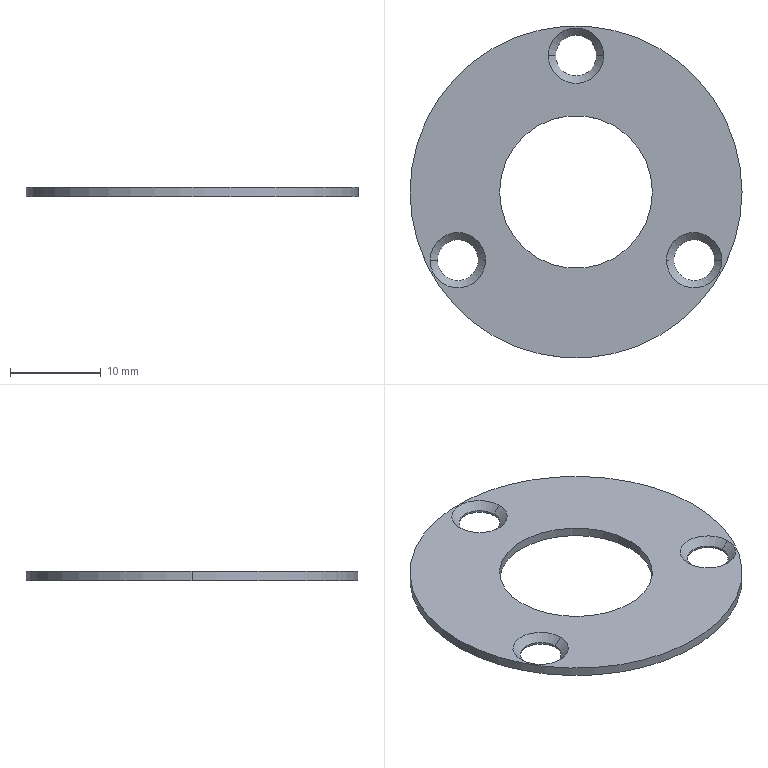Part | SolidWorks | features Chamfer 1, Extrusion 1 | 1 solid | 18 faces | box 36.5 x 36.5 x 1 mm | volume 761.783 mm3 | cylinder 10 | cone 6 | plane 2 | commonest cylinder face diameters 4.5 x6 16.8 x2 36.5 x2
STEP:
#1=CARTESIAN_POINT('',(-2.25,15.,0.2));
#2=VERTEX_POINT('',#1);
#3=CARTESIAN_POINT('',(2.25,15.,0.2));
#4=VERTEX_POINT('',#3);
#5=CARTESIAN_POINT('',(0.,15.,0.2));
#6=DIRECTION('',(0.,0.,1.));
#7=DIRECTION('',(1.,0.,0.));
#8=AXIS2_PLACEMENT_3D('',#5,#6,#7);
#9=CIRCLE('',#8,2.25);
#10=EDGE_CURVE('',#2,#4,#9,.T.);
#11=ORIENTED_EDGE('',*,*,#10,.F.);
#12=CARTESIAN_POINT('',(-3.05,15.,1.));
#13=VERTEX_POINT('',#12);
#14=CARTESIAN_POINT('',(-2.25,15.,0.2));
#15=DIRECTION('',(-0.7071,0.,0.7071));
#16=VECTOR('',#15,1000.);
#17=LINE('',#14,#16);
#18=EDGE_CURVE('',#2,#13,#17,.T.);
#19=ORIENTED_EDGE('',*,*,#18,.T.);
#20=CARTESIAN_POINT('',(3.05,15.,1.));
#21=VERTEX_POINT('',#20);
#22=CARTESIAN_POINT('',(0.,15.,1.));
#23=DIRECTION('',(0.,0.,-1.));
#24=DIRECTION('',(1.,0.,0.));
#25=AXIS2_PLACEMENT_3D('',#22,#23,#24);
#26=CIRCLE('',#25,3.05);
#27=EDGE_CURVE('',#21,#13,#26,.T.);
#28=ORIENTED_EDGE('',*,*,#27,.F.);
#29=CARTESIAN_POINT('',(2.25,15.,0.2));
#30=DIRECTION('',(0.7071,0.,0.7071));
#31=VECTOR('',#30,1000.);
#32=LINE('',#29,#31);
#33=EDGE_CURVE('',#4,#21,#32,.T.);
#34=ORIENTED_EDGE('',*,*,#33,.F.);
#35=EDGE_LOOP('',(#11,#19,#28,#34));
#36=FACE_OUTER_BOUND('',#35,.T.);
#37=CARTESIAN_POINT('',(0.,15.,0.2));
#38=DIRECTION('',(0.,0.,1.));
#39=DIRECTION('',(1.,0.,0.));
#40=AXIS2_PLACEMENT_3D('',#37,#38,#39);
#41=CONICAL_SURFACE('',#40,2.25,0.7854);
#42=ADVANCED_FACE('',(#36),#41,.F.);
#43=CARTESIAN_POINT('',(-15.24,-7.5,0.2));
#44=VERTEX_POINT('',#43);
#45=CARTESIAN_POINT('',(-10.74,-7.5,0.2));
#46=VERTEX_POINT('',#45);
#47=CARTESIAN_POINT('',(-12.99,-7.5,0.2));
#48=DIRECTION('',(0.,0.,1.));
#49=DIRECTION('',(1.,0.,0.));
#50=AXIS2_PLACEMENT_3D('',#47,#48,#49);
#51=CIRCLE('',#50,2.25);
#52=EDGE_CURVE('',#44,#46,#51,.T.);
#53=ORIENTED_EDGE('',*,*,#52,.F.);
#54=CARTESIAN_POINT('',(-16.04,-7.5,1.));
#55=VERTEX_POINT('',#54);
#56=CARTESIAN_POINT('',(-15.24,-7.5,0.2));
#57=DIRECTION('',(-0.7071,0.,0.7071));
#58=VECTOR('',#57,1000.);
#59=LINE('',#56,#58);
#60=EDGE_CURVE('',#44,#55,#59,.T.);
#61=ORIENTED_EDGE('',*,*,#60,.T.);
#62=CARTESIAN_POINT('',(-9.94,-7.5,1.));
#63=VERTEX_POINT('',#62);
#64=CARTESIAN_POINT('',(-12.99,-7.5,1.));
#65=DIRECTION('',(0.,0.,-1.));
#66=DIRECTION('',(1.,0.,0.));
#67=AXIS2_PLACEMENT_3D('',#64,#65,#66);
#68=CIRCLE('',#67,3.05);
#69=EDGE_CURVE('',#63,#55,#68,.T.);
#70=ORIENTED_EDGE('',*,*,#69,.F.);
#71=CARTESIAN_POINT('',(-10.74,-7.5,0.2));
#72=DIRECTION('',(0.7071,0.,0.7071));
#73=VECTOR('',#72,1000.);
#74=LINE('',#71,#73);
#75=EDGE_CURVE('',#46,#63,#74,.T.);
#76=ORIENTED_EDGE('',*,*,#75,.F.);
#77=EDGE_LOOP('',(#53,#61,#70,#76));
#78=FACE_OUTER_BOUND('',#77,.T.);
#79=CARTESIAN_POINT('',(-12.99,-7.5,0.2));
#80=DIRECTION('',(0.,0.,1.));
#81=DIRECTION('',(1.,0.,0.));
#82=AXIS2_PLACEMENT_3D('',#79,#80,#81);
#83=CONICAL_SURFACE('',#82,2.25,0.7854);
#84=ADVANCED_FACE('',(#78),#83,.F.);
#85=CARTESIAN_POINT('',(10.74,-7.5,0.2));
#86=VERTEX_POINT('',#85);
#87=CARTESIAN_POINT('',(15.24,-7.5,0.2));
#88=VERTEX_POINT('',#87);
#89=CARTESIAN_POINT('',(12.99,-7.5,0.2));
#90=DIRECTION('',(0.,0.,1.));
#91=DIRECTION('',(1.,0.,0.));
#92=AXIS2_PLACEMENT_3D('',#89,#90,#91);
#93=CIRCLE('',#92,2.25);
#94=EDGE_CURVE('',#86,#88,#93,.T.);
#95=ORIENTED_EDGE('',*,*,#94,.F.);
#96=CARTESIAN_POINT('',(9.94,-7.5,1.));
#97=VERTEX_POINT('',#96);
#98=CARTESIAN_POINT('',(10.74,-7.5,0.2));
#99=DIRECTION('',(-0.7071,0.,0.7071));
#100=VECTOR('',#99,1000.);
#101=LINE('',#98,#100);
#102=EDGE_CURVE('',#86,#97,#101,.T.);
#103=ORIENTED_EDGE('',*,*,#102,.T.);
#104=CARTESIAN_POINT('',(16.04,-7.5,1.));
#105=VERTEX_POINT('',#104);
#106=CARTESIAN_POINT('',(12.99,-7.5,1.));
#107=DIRECTION('',(0.,0.,-1.));
#108=DIRECTION('',(1.,0.,0.));
#109=AXIS2_PLACEMENT_3D('',#106,#107,#108);
#110=CIRCLE('',#109,3.05);
#111=EDGE_CURVE('',#105,#97,#110,.T.);
#112=ORIENTED_EDGE('',*,*,#111,.F.);
#113=CARTESIAN_POINT('',(15.24,-7.5,0.2));
#114=DIRECTION('',(0.7071,0.,0.7071));
#115=VECTOR('',#114,1000.);
#116=LINE('',#113,#115);
#117=EDGE_CURVE('',#88,#105,#116,.T.);
#118=ORIENTED_EDGE('',*,*,#117,.F.);
#119=EDGE_LOOP('',(#95,#103,#112,#118));
#120=FACE_OUTER_BOUND('',#119,.T.);
#121=CARTESIAN_POINT('',(12.99,-7.5,0.2));
#122=DIRECTION('',(0.,0.,1.));
#123=DIRECTION('',(1.,0.,0.));
#124=AXIS2_PLACEMENT_3D('',#121,#122,#123);
#125=CONICAL_SURFACE('',#124,2.25,0.7854);
#126=ADVANCED_FACE('',(#120),#125,.F.);
#127=ORIENTED_EDGE('',*,*,#52,.T.);
#128=CARTESIAN_POINT('',(-10.74,-7.5,0.));
#129=VERTEX_POINT('',#128);
#130=CARTESIAN_POINT('',(-10.74,-7.5,1.));
#131=DIRECTION('',(0.,0.,-1.));
#132=VECTOR('',#131,1000.);
#133=LINE('',#130,#132);
#134=EDGE_CURVE('',#46,#129,#133,.T.);
#135=ORIENTED_EDGE('',*,*,#134,.T.);
#136=CARTESIAN_POINT('',(-15.24,-7.5,0.));
#137=VERTEX_POINT('',#136);
#138=CARTESIAN_POINT('',(-12.99,-7.5,0.));
#139=DIRECTION('',(0.,0.,1.));
#140=DIRECTION('',(1.,0.,0.));
#141=AXIS2_PLACEMENT_3D('',#138,#139,#140);
#142=CIRCLE('',#141,2.25);
#143=EDGE_CURVE('',#137,#129,#142,.T.);
#144=ORIENTED_EDGE('',*,*,#143,.F.);
#145=CARTESIAN_POINT('',(-15.24,-7.5,1.));
#146=DIRECTION('',(0.,0.,-1.));
#147=VECTOR('',#146,1000.);
#148=LINE('',#145,#147);
#149=EDGE_CURVE('',#44,#137,#148,.T.);
#150=ORIENTED_EDGE('',*,*,#149,.F.);
#151=EDGE_LOOP('',(#127,#135,#144,#150));
#152=FACE_OUTER_BOUND('',#151,.T.);
#153=CARTESIAN_POINT('',(-12.99,-7.5,1.));
#154=DIRECTION('',(0.,0.,-1.));
#155=DIRECTION('',(-1.,0.,0.));
#156=AXIS2_PLACEMENT_3D('',#153,#154,#155);
#157=CYLINDRICAL_SURFACE('',#156,2.25);
#158=ADVANCED_FACE('',(#152),#157,.F.);
#159=ORIENTED_EDGE('',*,*,#94,.T.);
#160=CARTESIAN_POINT('',(15.24,-7.5,0.));
#161=VERTEX_POINT('',#160);
#162=CARTESIAN_POINT('',(15.24,-7.5,1.));
#163=DIRECTION('',(0.,0.,-1.));
#164=VECTOR('',#163,1000.);
#165=LINE('',#162,#164);
#166=EDGE_CURVE('',#88,#161,#165,.T.);
#167=ORIENTED_EDGE('',*,*,#166,.T.);
#168=CARTESIAN_POINT('',(10.74,-7.5,0.));
#169=VERTEX_POINT('',#168);
#170=CARTESIAN_POINT('',(12.99,-7.5,0.));
#171=DIRECTION('',(0.,0.,1.));
#172=DIRECTION('',(1.,0.,0.));
#173=AXIS2_PLACEMENT_3D('',#170,#171,#172);
#174=CIRCLE('',#173,2.25);
#175=EDGE_CURVE('',#169,#161,#174,.T.);
#176=ORIENTED_EDGE('',*,*,#175,.F.);
#177=CARTESIAN_POINT('',(10.74,-7.5,1.));
#178=DIRECTION('',(0.,0.,-1.));
#179=VECTOR('',#178,1000.);
#180=LINE('',#177,#179);
#181=EDGE_CURVE('',#86,#169,#180,.T.);
#182=ORIENTED_EDGE('',*,*,#181,.F.);
#183=EDGE_LOOP('',(#159,#167,#176,#182));
#184=FACE_OUTER_BOUND('',#183,.T.);
#185=CARTESIAN_POINT('',(12.99,-7.5,1.));
#186=DIRECTION('',(0.,0.,-1.));
#187=DIRECTION('',(-1.,0.,0.));
#188=AXIS2_PLACEMENT_3D('',#185,#186,#187);
#189=CYLINDRICAL_SURFACE('',#188,2.25);
#190=ADVANCED_FACE('',(#184),#189,.F.);
#191=ORIENTED_EDGE('',*,*,#10,.T.);
#192=CARTESIAN_POINT('',(2.25,15.,0.));
#193=VERTEX_POINT('',#192);
#194=CARTESIAN_POINT('',(2.25,15.,1.));
#195=DIRECTION('',(0.,0.,-1.));
#196=VECTOR('',#195,1000.);
#197=LINE('',#194,#196);
#198=EDGE_CURVE('',#4,#193,#197,.T.);
#199=ORIENTED_EDGE('',*,*,#198,.T.);
#200=CARTESIAN_POINT('',(-2.25,15.,0.));
#201=VERTEX_POINT('',#200);
#202=CARTESIAN_POINT('',(0.,15.,0.));
#203=DIRECTION('',(0.,0.,1.));
#204=DIRECTION('',(1.,0.,0.));
#205=AXIS2_PLACEMENT_3D('',#202,#203,#204);
#206=CIRCLE('',#205,2.25);
#207=EDGE_CURVE('',#201,#193,#206,.T.);
#208=ORIENTED_EDGE('',*,*,#207,.F.);
#209=CARTESIAN_POINT('',(-2.25,15.,1.));
#210=DIRECTION('',(0.,0.,-1.));
#211=VECTOR('',#210,1000.);
#212=LINE('',#209,#211);
#213=EDGE_CURVE('',#2,#201,#212,.T.);
#214=ORIENTED_EDGE('',*,*,#213,.F.);
#215=EDGE_LOOP('',(#191,#199,#208,#214));
#216=FACE_OUTER_BOUND('',#215,.T.);
#217=CARTESIAN_POINT('',(0.,15.,1.));
#218=DIRECTION('',(0.,0.,-1.));
#219=DIRECTION('',(-1.,0.,0.));
#220=AXIS2_PLACEMENT_3D('',#217,#218,#219);
#221=CYLINDRICAL_SURFACE('',#220,2.25);
#222=ADVANCED_FACE('',(#216),#221,.F.);
#223=CARTESIAN_POINT('',(-8.4,0.,1.));
#224=VERTEX_POINT('',#223);
#225=CARTESIAN_POINT('',(8.4,0.,1.));
#226=VERTEX_POINT('',#225);
#227=CARTESIAN_POINT('',(0.,0.,1.));
#228=DIRECTION('',(0.,0.,1.));
#229=DIRECTION('',(1.,0.,0.));
#230=AXIS2_PLACEMENT_3D('',#227,#228,#229);
#231=CIRCLE('',#230,8.4);
#232=EDGE_CURVE('',#224,#226,#231,.T.);
#233=ORIENTED_EDGE('',*,*,#232,.T.);
#234=CARTESIAN_POINT('',(8.4,0.,0.));
#235=VERTEX_POINT('',#234);
#236=CARTESIAN_POINT('',(8.4,0.,1.));
#237=DIRECTION('',(0.,0.,-1.));
#238=VECTOR('',#237,1000.);
#239=LINE('',#236,#238);
#240=EDGE_CURVE('',#226,#235,#239,.T.);
#241=ORIENTED_EDGE('',*,*,#240,.T.);
#242=CARTESIAN_POINT('',(-8.4,0.,0.));
#243=VERTEX_POINT('',#242);
#244=CARTESIAN_POINT('',(0.,0.,0.));
#245=DIRECTION('',(0.,0.,1.));
#246=DIRECTION('',(1.,0.,0.));
#247=AXIS2_PLACEMENT_3D('',#244,#245,#246);
#248=CIRCLE('',#247,8.4);
#249=EDGE_CURVE('',#243,#235,#248,.T.);
#250=ORIENTED_EDGE('',*,*,#249,.F.);
#251=CARTESIAN_POINT('',(-8.4,0.,1.));
#252=DIRECTION('',(0.,0.,-1.));
#253=VECTOR('',#252,1000.);
#254=LINE('',#251,#253);
#255=EDGE_CURVE('',#224,#243,#254,.T.);
#256=ORIENTED_EDGE('',*,*,#255,.F.);
#257=EDGE_LOOP('',(#233,#241,#250,#256));
#258=FACE_OUTER_BOUND('',#257,.T.);
#259=CARTESIAN_POINT('',(0.,0.,1.));
#260=DIRECTION('',(0.,0.,-1.));
#261=DIRECTION('',(-1.,0.,0.));
#262=AXIS2_PLACEMENT_3D('',#259,#260,#261);
#263=CYLINDRICAL_SURFACE('',#262,8.4);
#264=ADVANCED_FACE('',(#258),#263,.F.);
#265=CARTESIAN_POINT('',(18.25,0.,1.));
#266=VERTEX_POINT('',#265);
#267=CARTESIAN_POINT('',(-18.25,0.,1.));
#268=VERTEX_POINT('',#267);
#269=CARTESIAN_POINT('',(0.,0.,1.));
#270=DIRECTION('',(0.,0.,1.));
#271=DIRECTION('',(1.,0.,0.));
#272=AXIS2_PLACEMENT_3D('',#269,#270,#271);
#273=CIRCLE('',#272,18.25);
#274=EDGE_CURVE('',#266,#268,#273,.T.);
#275=ORIENTED_EDGE('',*,*,#274,.F.);
#276=CARTESIAN_POINT('',(18.25,0.,0.));
#277=VERTEX_POINT('',#276);
#278=CARTESIAN_POINT('',(18.25,0.,1.));
#279=DIRECTION('',(0.,0.,-1.));
#280=VECTOR('',#279,1000.);
#281=LINE('',#278,#280);
#282=EDGE_CURVE('',#266,#277,#281,.T.);
#283=ORIENTED_EDGE('',*,*,#282,.T.);
#284=CARTESIAN_POINT('',(-18.25,0.,0.));
#285=VERTEX_POINT('',#284);
#286=CARTESIAN_POINT('',(0.,0.,0.));
#287=DIRECTION('',(0.,0.,1.));
#288=DIRECTION('',(1.,0.,0.));
#289=AXIS2_PLACEMENT_3D('',#286,#287,#288);
#290=CIRCLE('',#289,18.25);
#291=EDGE_CURVE('',#277,#285,#290,.T.);
#292=ORIENTED_EDGE('',*,*,#291,.T.);
#293=CARTESIAN_POINT('',(-18.25,0.,1.));
#294=DIRECTION('',(0.,0.,-1.));
#295=VECTOR('',#294,1000.);
#296=LINE('',#293,#295);
#297=EDGE_CURVE('',#268,#285,#296,.T.);
#298=ORIENTED_EDGE('',*,*,#297,.F.);
#299=EDGE_LOOP('',(#275,#283,#292,#298));
#300=FACE_OUTER_BOUND('',#299,.T.);
#301=CARTESIAN_POINT('',(0.,0.,1.));
#302=DIRECTION('',(0.,0.,-1.));
#303=DIRECTION('',(-1.,0.,0.));
#304=AXIS2_PLACEMENT_3D('',#301,#302,#303);
#305=CYLINDRICAL_SURFACE('',#304,18.25);
#306=ADVANCED_FACE('',(#300),#305,.T.);
#307=ORIENTED_EDGE('',*,*,#111,.T.);
#308=CARTESIAN_POINT('',(12.99,-7.5,1.));
#309=DIRECTION('',(0.,0.,-1.));
#310=DIRECTION('',(1.,0.,0.));
#311=AXIS2_PLACEMENT_3D('',#308,#309,#310);
#312=CIRCLE('',#311,3.05);
#313=EDGE_CURVE('',#97,#105,#312,.T.);
#314=ORIENTED_EDGE('',*,*,#313,.T.);
#315=EDGE_LOOP('',(#307,#314));
#316=FACE_BOUND('',#315,.T.);
#317=ORIENTED_EDGE('',*,*,#69,.T.);
#318=CARTESIAN_POINT('',(-12.99,-7.5,1.));
#319=DIRECTION('',(0.,0.,-1.));
#320=DIRECTION('',(1.,0.,0.));
#321=AXIS2_PLACEMENT_3D('',#318,#319,#320);
#322=CIRCLE('',#321,3.05);
#323=EDGE_CURVE('',#55,#63,#322,.T.);
#324=ORIENTED_EDGE('',*,*,#323,.T.);
#325=EDGE_LOOP('',(#317,#324));
#326=FACE_BOUND('',#325,.T.);
#327=ORIENTED_EDGE('',*,*,#27,.T.);
#328=CARTESIAN_POINT('',(0.,15.,1.));
#329=DIRECTION('',(0.,0.,-1.));
#330=DIRECTION('',(1.,0.,0.));
#331=AXIS2_PLACEMENT_3D('',#328,#329,#330);
#332=CIRCLE('',#331,3.05);
#333=EDGE_CURVE('',#13,#21,#332,.T.);
#334=ORIENTED_EDGE('',*,*,#333,.T.);
#335=EDGE_LOOP('',(#327,#334));
#336=FACE_BOUND('',#335,.T.);
#337=ORIENTED_EDGE('',*,*,#232,.F.);
#338=CARTESIAN_POINT('',(0.,0.,1.));
#339=DIRECTION('',(0.,0.,1.));
#340=DIRECTION('',(1.,0.,0.));
#341=AXIS2_PLACEMENT_3D('',#338,#339,#340);
#342=CIRCLE('',#341,8.4);
#343=EDGE_CURVE('',#226,#224,#342,.T.);
#344=ORIENTED_EDGE('',*,*,#343,.F.);
#345=EDGE_LOOP('',(#337,#344));
#346=FACE_BOUND('',#345,.T.);
#347=CARTESIAN_POINT('',(0.,0.,1.));
#348=DIRECTION('',(0.,0.,1.));
#349=DIRECTION('',(1.,0.,0.));
#350=AXIS2_PLACEMENT_3D('',#347,#348,#349);
#351=CIRCLE('',#350,18.25);
#352=EDGE_CURVE('',#268,#266,#351,.T.);
#353=ORIENTED_EDGE('',*,*,#352,.T.);
#354=ORIENTED_EDGE('',*,*,#274,.T.);
#355=EDGE_LOOP('',(#353,#354));
#356=FACE_OUTER_BOUND('',#355,.T.);
#357=CARTESIAN_POINT('',(0.,0.,1.));
#358=DIRECTION('',(0.,0.,1.));
#359=DIRECTION('',(1.,0.,0.));
#360=AXIS2_PLACEMENT_3D('',#357,#358,#359);
#361=PLANE('',#360);
#362=ADVANCED_FACE('',(#316,#326,#336,#346,#356),#361,.T.);
#363=ORIENTED_EDGE('',*,*,#175,.T.);
#364=CARTESIAN_POINT('',(12.99,-7.5,0.));
#365=DIRECTION('',(0.,0.,1.));
#366=DIRECTION('',(1.,0.,0.));
#367=AXIS2_PLACEMENT_3D('',#364,#365,#366);
#368=CIRCLE('',#367,2.25);
#369=EDGE_CURVE('',#161,#169,#368,.T.);
#370=ORIENTED_EDGE('',*,*,#369,.T.);
#371=EDGE_LOOP('',(#363,#370));
#372=FACE_BOUND('',#371,.T.);
#373=ORIENTED_EDGE('',*,*,#249,.T.);
#374=CARTESIAN_POINT('',(0.,0.,0.));
#375=DIRECTION('',(0.,0.,1.));
#376=DIRECTION('',(1.,0.,0.));
#377=AXIS2_PLACEMENT_3D('',#374,#375,#376);
#378=CIRCLE('',#377,8.4);
#379=EDGE_CURVE('',#235,#243,#378,.T.);
#380=ORIENTED_EDGE('',*,*,#379,.T.);
#381=EDGE_LOOP('',(#373,#380));
#382=FACE_BOUND('',#381,.T.);
#383=CARTESIAN_POINT('',(0.,0.,0.));
#384=DIRECTION('',(0.,0.,1.));
#385=DIRECTION('',(1.,0.,0.));
#386=AXIS2_PLACEMENT_3D('',#383,#384,#385);
#387=CIRCLE('',#386,18.25);
#388=EDGE_CURVE('',#285,#277,#387,.T.);
#389=ORIENTED_EDGE('',*,*,#388,.F.);
#390=ORIENTED_EDGE('',*,*,#291,.F.);
#391=EDGE_LOOP('',(#389,#390));
#392=FACE_OUTER_BOUND('',#391,.T.);
#393=ORIENTED_EDGE('',*,*,#207,.T.);
#394=CARTESIAN_POINT('',(0.,15.,0.));
#395=DIRECTION('',(0.,0.,1.));
#396=DIRECTION('',(1.,0.,0.));
#397=AXIS2_PLACEMENT_3D('',#394,#395,#396);
#398=CIRCLE('',#397,2.25);
#399=EDGE_CURVE('',#193,#201,#398,.T.);
#400=ORIENTED_EDGE('',*,*,#399,.T.);
#401=EDGE_LOOP('',(#393,#400));
#402=FACE_BOUND('',#401,.T.);
#403=ORIENTED_EDGE('',*,*,#143,.T.);
#404=CARTESIAN_POINT('',(-12.99,-7.5,0.));
#405=DIRECTION('',(0.,0.,1.));
#406=DIRECTION('',(1.,0.,0.));
#407=AXIS2_PLACEMENT_3D('',#404,#405,#406);
#408=CIRCLE('',#407,2.25);
#409=EDGE_CURVE('',#129,#137,#408,.T.);
#410=ORIENTED_EDGE('',*,*,#409,.T.);
#411=EDGE_LOOP('',(#403,#410));
#412=FACE_BOUND('',#411,.T.);
#413=CARTESIAN_POINT('',(0.,0.,0.));
#414=DIRECTION('',(0.,0.,1.));
#415=DIRECTION('',(1.,0.,0.));
#416=AXIS2_PLACEMENT_3D('',#413,#414,#415);
#417=PLANE('',#416);
#418=ADVANCED_FACE('',(#372,#382,#392,#402,#412),#417,.F.);
#419=ORIENTED_EDGE('',*,*,#282,.F.);
#420=ORIENTED_EDGE('',*,*,#352,.F.);
#421=ORIENTED_EDGE('',*,*,#297,.T.);
#422=ORIENTED_EDGE('',*,*,#388,.T.);
#423=EDGE_LOOP('',(#419,#420,#421,#422));
#424=FACE_OUTER_BOUND('',#423,.T.);
#425=CARTESIAN_POINT('',(0.,0.,1.));
#426=DIRECTION('',(0.,0.,-1.));
#427=DIRECTION('',(-1.,0.,0.));
#428=AXIS2_PLACEMENT_3D('',#425,#426,#427);
#429=CYLINDRICAL_SURFACE('',#428,18.25);
#430=ADVANCED_FACE('',(#424),#429,.T.);
#431=ORIENTED_EDGE('',*,*,#240,.F.);
#432=ORIENTED_EDGE('',*,*,#343,.T.);
#433=ORIENTED_EDGE('',*,*,#255,.T.);
#434=ORIENTED_EDGE('',*,*,#379,.F.);
#435=EDGE_LOOP('',(#431,#432,#433,#434));
#436=FACE_OUTER_BOUND('',#435,.T.);
#437=CARTESIAN_POINT('',(0.,0.,1.));
#438=DIRECTION('',(0.,0.,-1.));
#439=DIRECTION('',(-1.,0.,0.));
#440=AXIS2_PLACEMENT_3D('',#437,#438,#439);
#441=CYLINDRICAL_SURFACE('',#440,8.4);
#442=ADVANCED_FACE('',(#436),#441,.F.);
#443=ORIENTED_EDGE('',*,*,#198,.F.);
#444=CARTESIAN_POINT('',(0.,15.,0.2));
#445=DIRECTION('',(0.,0.,1.));
#446=DIRECTION('',(1.,0.,0.));
#447=AXIS2_PLACEMENT_3D('',#444,#445,#446);
#448=CIRCLE('',#447,2.25);
#449=EDGE_CURVE('',#4,#2,#448,.T.);
#450=ORIENTED_EDGE('',*,*,#449,.T.);
#451=ORIENTED_EDGE('',*,*,#213,.T.);
#452=ORIENTED_EDGE('',*,*,#399,.F.);
#453=EDGE_LOOP('',(#443,#450,#451,#452));
#454=FACE_OUTER_BOUND('',#453,.T.);
#455=CARTESIAN_POINT('',(0.,15.,1.));
#456=DIRECTION('',(0.,0.,-1.));
#457=DIRECTION('',(-1.,0.,0.));
#458=AXIS2_PLACEMENT_3D('',#455,#456,#457);
#459=CYLINDRICAL_SURFACE('',#458,2.25);
#460=ADVANCED_FACE('',(#454),#459,.F.);
#461=ORIENTED_EDGE('',*,*,#166,.F.);
#462=CARTESIAN_POINT('',(12.99,-7.5,0.2));
#463=DIRECTION('',(0.,0.,1.));
#464=DIRECTION('',(1.,0.,0.));
#465=AXIS2_PLACEMENT_3D('',#462,#463,#464);
#466=CIRCLE('',#465,2.25);
#467=EDGE_CURVE('',#88,#86,#466,.T.);
#468=ORIENTED_EDGE('',*,*,#467,.T.);
#469=ORIENTED_EDGE('',*,*,#181,.T.);
#470=ORIENTED_EDGE('',*,*,#369,.F.);
#471=EDGE_LOOP('',(#461,#468,#469,#470));
#472=FACE_OUTER_BOUND('',#471,.T.);
#473=CARTESIAN_POINT('',(12.99,-7.5,1.));
#474=DIRECTION('',(0.,0.,-1.));
#475=DIRECTION('',(-1.,0.,0.));
#476=AXIS2_PLACEMENT_3D('',#473,#474,#475);
#477=CYLINDRICAL_SURFACE('',#476,2.25);
#478=ADVANCED_FACE('',(#472),#477,.F.);
#479=ORIENTED_EDGE('',*,*,#134,.F.);
#480=CARTESIAN_POINT('',(-12.99,-7.5,0.2));
#481=DIRECTION('',(0.,0.,1.));
#482=DIRECTION('',(1.,0.,0.));
#483=AXIS2_PLACEMENT_3D('',#480,#481,#482);
#484=CIRCLE('',#483,2.25);
#485=EDGE_CURVE('',#46,#44,#484,.T.);
#486=ORIENTED_EDGE('',*,*,#485,.T.);
#487=ORIENTED_EDGE('',*,*,#149,.T.);
#488=ORIENTED_EDGE('',*,*,#409,.F.);
#489=EDGE_LOOP('',(#479,#486,#487,#488));
#490=FACE_OUTER_BOUND('',#489,.T.);
#491=CARTESIAN_POINT('',(-12.99,-7.5,1.));
#492=DIRECTION('',(0.,0.,-1.));
#493=DIRECTION('',(-1.,0.,0.));
#494=AXIS2_PLACEMENT_3D('',#491,#492,#493);
#495=CYLINDRICAL_SURFACE('',#494,2.25);
#496=ADVANCED_FACE('',(#490),#495,.F.);
#497=ORIENTED_EDGE('',*,*,#102,.F.);
#498=ORIENTED_EDGE('',*,*,#467,.F.);
#499=ORIENTED_EDGE('',*,*,#117,.T.);
#500=ORIENTED_EDGE('',*,*,#313,.F.);
#501=EDGE_LOOP('',(#497,#498,#499,#500));
#502=FACE_OUTER_BOUND('',#501,.T.);
#503=CARTESIAN_POINT('',(12.99,-7.5,0.2));
#504=DIRECTION('',(0.,0.,1.));
#505=DIRECTION('',(1.,0.,0.));
#506=AXIS2_PLACEMENT_3D('',#503,#504,#505);
#507=CONICAL_SURFACE('',#506,2.25,0.7854);
#508=ADVANCED_FACE('',(#502),#507,.F.);
#509=ORIENTED_EDGE('',*,*,#60,.F.);
#510=ORIENTED_EDGE('',*,*,#485,.F.);
#511=ORIENTED_EDGE('',*,*,#75,.T.);
#512=ORIENTED_EDGE('',*,*,#323,.F.);
#513=EDGE_LOOP('',(#509,#510,#511,#512));
#514=FACE_OUTER_BOUND('',#513,.T.);
#515=CARTESIAN_POINT('',(-12.99,-7.5,0.2));
#516=DIRECTION('',(0.,0.,1.));
#517=DIRECTION('',(1.,0.,0.));
#518=AXIS2_PLACEMENT_3D('',#515,#516,#517);
#519=CONICAL_SURFACE('',#518,2.25,0.7854);
#520=ADVANCED_FACE('',(#514),#519,.F.);
#521=ORIENTED_EDGE('',*,*,#18,.F.);
#522=ORIENTED_EDGE('',*,*,#449,.F.);
#523=ORIENTED_EDGE('',*,*,#33,.T.);
#524=ORIENTED_EDGE('',*,*,#333,.F.);
#525=EDGE_LOOP('',(#521,#522,#523,#524));
#526=FACE_OUTER_BOUND('',#525,.T.);
#527=CARTESIAN_POINT('',(0.,15.,0.2));
#528=DIRECTION('',(0.,0.,1.));
#529=DIRECTION('',(1.,0.,0.));
#530=AXIS2_PLACEMENT_3D('',#527,#528,#529);
#531=CONICAL_SURFACE('',#530,2.25,0.7854);
#532=ADVANCED_FACE('',(#526),#531,.F.);
#533=CLOSED_SHELL('',(#42,#84,#126,#158,#190,#222,#264,#306,#362,#418,#430,#442,#460,#478,#496,#508,#520,#532));
#534=MANIFOLD_SOLID_BREP('',#533);
#535=CARTESIAN_POINT('',(0.,0.,0.));
#536=DIRECTION('',(0.,0.,1.));
#537=DIRECTION('',(1.,0.,0.));
#538=AXIS2_PLACEMENT_3D('',#535,#536,#537);
#539=(LENGTH_UNIT()NAMED_UNIT(*)SI_UNIT(.MILLI.,.METRE.));
#540=UNCERTAINTY_MEASURE_WITH_UNIT(LENGTH_MEASURE(0.00001),#539,'','');
#541=(NAMED_UNIT(*)PLANE_ANGLE_UNIT()SI_UNIT($,.RADIAN.));
#542=(NAMED_UNIT(*)SI_UNIT($,.STERADIAN.)SOLID_ANGLE_UNIT());
#543=(GEOMETRIC_REPRESENTATION_CONTEXT(3)GLOBAL_UNCERTAINTY_ASSIGNED_CONTEXT((#540))GLOBAL_UNIT_ASSIGNED_CONTEXT((#539,#541,#542))REPRESENTATION_CONTEXT('',''));
#544=ADVANCED_BREP_SHAPE_REPRESENTATION('',(#534,#538),#543);